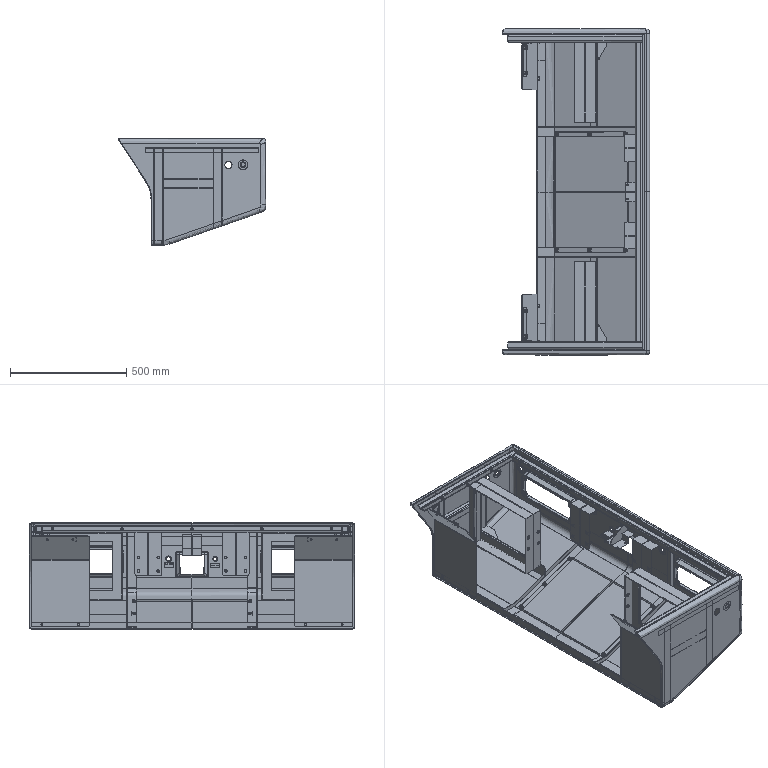Part | NX | features BREP 93 | 50 solids | 2684 faces | box 632.819 x 1400 x 457 mm | volume 1445450 mm3 | plane 1323 | cylinder 803 | spline 288 | cone 262 | torus 6 | sphere 2 | commonest cylinder face diameters 8 x168 10 x122 13 x68 11 x52 20 x44 16 x36